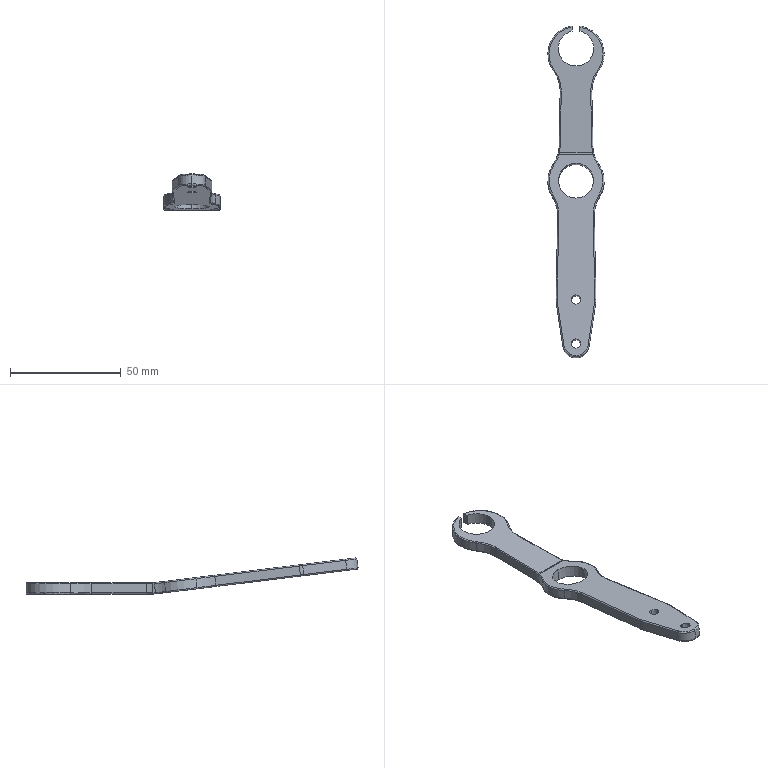Part | SolidWorks | features BaseBody 1 | 1 solid | 103 faces | box 25.4 x 149.639 x 16.267 mm | volume 11045 mm3 | spline 48 | cylinder 43 | plane 12 | commonest cylinder face diameters 1.016 x14 30.48 x9 25.4 x5 4.166 x4 16 x3 12 x2